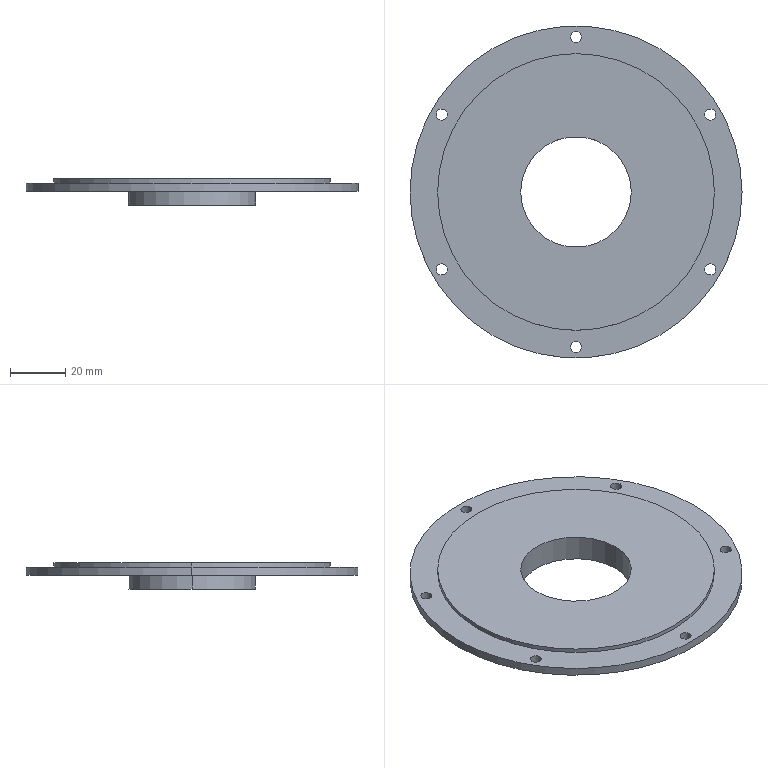Part | SolidWorks | features ICE 1, Revolution 1 | 1 solid | 24 faces | box 120 x 120 x 9.5 mm | volume 41855 mm3 | cylinder 20 | plane 4 | commonest cylinder face diameters 4 x12 40 x2 46 x2 100 x2 120 x2
STEP:
#1=CARTESIAN_POINT('',(2.,56.,-1.5));
#2=VERTEX_POINT('',#1);
#3=CARTESIAN_POINT('',(-2.,56.,-1.5));
#4=VERTEX_POINT('',#3);
#5=CARTESIAN_POINT('',(0.,56.,-1.5));
#6=DIRECTION('',(0.,0.,-1.));
#7=DIRECTION('',(-1.,0.,0.));
#8=AXIS2_PLACEMENT_3D('',#5,#6,#7);
#9=CIRCLE('',#8,2.);
#10=EDGE_CURVE('',#2,#4,#9,.T.);
#11=ORIENTED_EDGE('',*,*,#10,.F.);
#12=CARTESIAN_POINT('',(2.,56.,-4.5));
#13=VERTEX_POINT('',#12);
#14=CARTESIAN_POINT('',(2.,56.,5.5));
#15=DIRECTION('',(0.,0.,-1.));
#16=VECTOR('',#15,1000.);
#17=LINE('',#14,#16);
#18=EDGE_CURVE('',#2,#13,#17,.T.);
#19=ORIENTED_EDGE('',*,*,#18,.T.);
#20=CARTESIAN_POINT('',(-2.,56.,-4.5));
#21=VERTEX_POINT('',#20);
#22=CARTESIAN_POINT('',(0.,56.,-4.5));
#23=DIRECTION('',(0.,0.,-1.));
#24=DIRECTION('',(-1.,0.,0.));
#25=AXIS2_PLACEMENT_3D('',#22,#23,#24);
#26=CIRCLE('',#25,2.);
#27=EDGE_CURVE('',#13,#21,#26,.T.);
#28=ORIENTED_EDGE('',*,*,#27,.T.);
#29=CARTESIAN_POINT('',(-2.,56.,5.5));
#30=DIRECTION('',(0.,0.,-1.));
#31=VECTOR('',#30,1000.);
#32=LINE('',#29,#31);
#33=EDGE_CURVE('',#4,#21,#32,.T.);
#34=ORIENTED_EDGE('',*,*,#33,.F.);
#35=EDGE_LOOP('',(#11,#19,#28,#34));
#36=FACE_OUTER_BOUND('',#35,.T.);
#37=CARTESIAN_POINT('',(0.,56.,5.5));
#38=DIRECTION('',(0.,0.,-1.));
#39=DIRECTION('',(-1.,0.,0.));
#40=AXIS2_PLACEMENT_3D('',#37,#38,#39);
#41=CYLINDRICAL_SURFACE('',#40,2.);
#42=ADVANCED_FACE('',(#36),#41,.F.);
#43=CARTESIAN_POINT('',(-46.497,28.,-1.5));
#44=VERTEX_POINT('',#43);
#45=CARTESIAN_POINT('',(-50.497,28.,-1.5));
#46=VERTEX_POINT('',#45);
#47=CARTESIAN_POINT('',(-48.497,28.,-1.5));
#48=DIRECTION('',(0.,0.,-1.));
#49=DIRECTION('',(-1.,0.,0.));
#50=AXIS2_PLACEMENT_3D('',#47,#48,#49);
#51=CIRCLE('',#50,2.);
#52=EDGE_CURVE('',#44,#46,#51,.T.);
#53=ORIENTED_EDGE('',*,*,#52,.F.);
#54=CARTESIAN_POINT('',(-46.497,28.,-4.5));
#55=VERTEX_POINT('',#54);
#56=CARTESIAN_POINT('',(-46.497,28.,5.5));
#57=DIRECTION('',(0.,0.,-1.));
#58=VECTOR('',#57,1000.);
#59=LINE('',#56,#58);
#60=EDGE_CURVE('',#44,#55,#59,.T.);
#61=ORIENTED_EDGE('',*,*,#60,.T.);
#62=CARTESIAN_POINT('',(-50.497,28.,-4.5));
#63=VERTEX_POINT('',#62);
#64=CARTESIAN_POINT('',(-48.497,28.,-4.5));
#65=DIRECTION('',(0.,0.,-1.));
#66=DIRECTION('',(-1.,0.,0.));
#67=AXIS2_PLACEMENT_3D('',#64,#65,#66);
#68=CIRCLE('',#67,2.);
#69=EDGE_CURVE('',#55,#63,#68,.T.);
#70=ORIENTED_EDGE('',*,*,#69,.T.);
#71=CARTESIAN_POINT('',(-50.497,28.,5.5));
#72=DIRECTION('',(0.,0.,-1.));
#73=VECTOR('',#72,1000.);
#74=LINE('',#71,#73);
#75=EDGE_CURVE('',#46,#63,#74,.T.);
#76=ORIENTED_EDGE('',*,*,#75,.F.);
#77=EDGE_LOOP('',(#53,#61,#70,#76));
#78=FACE_OUTER_BOUND('',#77,.T.);
#79=CARTESIAN_POINT('',(-48.497,28.,5.5));
#80=DIRECTION('',(0.,0.,-1.));
#81=DIRECTION('',(-1.,0.,0.));
#82=AXIS2_PLACEMENT_3D('',#79,#80,#81);
#83=CYLINDRICAL_SURFACE('',#82,2.);
#84=ADVANCED_FACE('',(#78),#83,.F.);
#85=CARTESIAN_POINT('',(-46.497,-28.,-1.5));
#86=VERTEX_POINT('',#85);
#87=CARTESIAN_POINT('',(-50.497,-28.,-1.5));
#88=VERTEX_POINT('',#87);
#89=CARTESIAN_POINT('',(-48.497,-28.,-1.5));
#90=DIRECTION('',(0.,0.,-1.));
#91=DIRECTION('',(-1.,0.,0.));
#92=AXIS2_PLACEMENT_3D('',#89,#90,#91);
#93=CIRCLE('',#92,2.);
#94=EDGE_CURVE('',#86,#88,#93,.T.);
#95=ORIENTED_EDGE('',*,*,#94,.F.);
#96=CARTESIAN_POINT('',(-46.497,-28.,-4.5));
#97=VERTEX_POINT('',#96);
#98=CARTESIAN_POINT('',(-46.497,-28.,5.5));
#99=DIRECTION('',(0.,0.,-1.));
#100=VECTOR('',#99,1000.);
#101=LINE('',#98,#100);
#102=EDGE_CURVE('',#86,#97,#101,.T.);
#103=ORIENTED_EDGE('',*,*,#102,.T.);
#104=CARTESIAN_POINT('',(-50.497,-28.,-4.5));
#105=VERTEX_POINT('',#104);
#106=CARTESIAN_POINT('',(-48.497,-28.,-4.5));
#107=DIRECTION('',(0.,0.,-1.));
#108=DIRECTION('',(-1.,0.,0.));
#109=AXIS2_PLACEMENT_3D('',#106,#107,#108);
#110=CIRCLE('',#109,2.);
#111=EDGE_CURVE('',#97,#105,#110,.T.);
#112=ORIENTED_EDGE('',*,*,#111,.T.);
#113=CARTESIAN_POINT('',(-50.497,-28.,5.5));
#114=DIRECTION('',(0.,0.,-1.));
#115=VECTOR('',#114,1000.);
#116=LINE('',#113,#115);
#117=EDGE_CURVE('',#88,#105,#116,.T.);
#118=ORIENTED_EDGE('',*,*,#117,.F.);
#119=EDGE_LOOP('',(#95,#103,#112,#118));
#120=FACE_OUTER_BOUND('',#119,.T.);
#121=CARTESIAN_POINT('',(-48.497,-28.,5.5));
#122=DIRECTION('',(0.,0.,-1.));
#123=DIRECTION('',(-1.,0.,0.));
#124=AXIS2_PLACEMENT_3D('',#121,#122,#123);
#125=CYLINDRICAL_SURFACE('',#124,2.);
#126=ADVANCED_FACE('',(#120),#125,.F.);
#127=CARTESIAN_POINT('',(2.,-56.,-1.5));
#128=VERTEX_POINT('',#127);
#129=CARTESIAN_POINT('',(-2.,-56.,-1.5));
#130=VERTEX_POINT('',#129);
#131=CARTESIAN_POINT('',(0.,-56.,-1.5));
#132=DIRECTION('',(0.,0.,-1.));
#133=DIRECTION('',(-1.,0.,0.));
#134=AXIS2_PLACEMENT_3D('',#131,#132,#133);
#135=CIRCLE('',#134,2.);
#136=EDGE_CURVE('',#128,#130,#135,.T.);
#137=ORIENTED_EDGE('',*,*,#136,.F.);
#138=CARTESIAN_POINT('',(2.,-56.,-4.5));
#139=VERTEX_POINT('',#138);
#140=CARTESIAN_POINT('',(2.,-56.,5.5));
#141=DIRECTION('',(0.,0.,-1.));
#142=VECTOR('',#141,1000.);
#143=LINE('',#140,#142);
#144=EDGE_CURVE('',#128,#139,#143,.T.);
#145=ORIENTED_EDGE('',*,*,#144,.T.);
#146=CARTESIAN_POINT('',(-2.,-56.,-4.5));
#147=VERTEX_POINT('',#146);
#148=CARTESIAN_POINT('',(0.,-56.,-4.5));
#149=DIRECTION('',(0.,0.,-1.));
#150=DIRECTION('',(-1.,0.,0.));
#151=AXIS2_PLACEMENT_3D('',#148,#149,#150);
#152=CIRCLE('',#151,2.);
#153=EDGE_CURVE('',#139,#147,#152,.T.);
#154=ORIENTED_EDGE('',*,*,#153,.T.);
#155=CARTESIAN_POINT('',(-2.,-56.,5.5));
#156=DIRECTION('',(0.,0.,-1.));
#157=VECTOR('',#156,1000.);
#158=LINE('',#155,#157);
#159=EDGE_CURVE('',#130,#147,#158,.T.);
#160=ORIENTED_EDGE('',*,*,#159,.F.);
#161=EDGE_LOOP('',(#137,#145,#154,#160));
#162=FACE_OUTER_BOUND('',#161,.T.);
#163=CARTESIAN_POINT('',(0.,-56.,5.5));
#164=DIRECTION('',(0.,0.,-1.));
#165=DIRECTION('',(-1.,0.,0.));
#166=AXIS2_PLACEMENT_3D('',#163,#164,#165);
#167=CYLINDRICAL_SURFACE('',#166,2.);
#168=ADVANCED_FACE('',(#162),#167,.F.);
#169=CARTESIAN_POINT('',(50.497,-28.,-1.5));
#170=VERTEX_POINT('',#169);
#171=CARTESIAN_POINT('',(46.497,-28.,-1.5));
#172=VERTEX_POINT('',#171);
#173=CARTESIAN_POINT('',(48.497,-28.,-1.5));
#174=DIRECTION('',(0.,0.,-1.));
#175=DIRECTION('',(-1.,0.,0.));
#176=AXIS2_PLACEMENT_3D('',#173,#174,#175);
#177=CIRCLE('',#176,2.);
#178=EDGE_CURVE('',#170,#172,#177,.T.);
#179=ORIENTED_EDGE('',*,*,#178,.F.);
#180=CARTESIAN_POINT('',(50.497,-28.,-4.5));
#181=VERTEX_POINT('',#180);
#182=CARTESIAN_POINT('',(50.497,-28.,5.5));
#183=DIRECTION('',(0.,0.,-1.));
#184=VECTOR('',#183,1000.);
#185=LINE('',#182,#184);
#186=EDGE_CURVE('',#170,#181,#185,.T.);
#187=ORIENTED_EDGE('',*,*,#186,.T.);
#188=CARTESIAN_POINT('',(46.497,-28.,-4.5));
#189=VERTEX_POINT('',#188);
#190=CARTESIAN_POINT('',(48.497,-28.,-4.5));
#191=DIRECTION('',(0.,0.,-1.));
#192=DIRECTION('',(-1.,0.,0.));
#193=AXIS2_PLACEMENT_3D('',#190,#191,#192);
#194=CIRCLE('',#193,2.);
#195=EDGE_CURVE('',#181,#189,#194,.T.);
#196=ORIENTED_EDGE('',*,*,#195,.T.);
#197=CARTESIAN_POINT('',(46.497,-28.,5.5));
#198=DIRECTION('',(0.,0.,-1.));
#199=VECTOR('',#198,1000.);
#200=LINE('',#197,#199);
#201=EDGE_CURVE('',#172,#189,#200,.T.);
#202=ORIENTED_EDGE('',*,*,#201,.F.);
#203=EDGE_LOOP('',(#179,#187,#196,#202));
#204=FACE_OUTER_BOUND('',#203,.T.);
#205=CARTESIAN_POINT('',(48.497,-28.,5.5));
#206=DIRECTION('',(0.,0.,-1.));
#207=DIRECTION('',(-1.,0.,0.));
#208=AXIS2_PLACEMENT_3D('',#205,#206,#207);
#209=CYLINDRICAL_SURFACE('',#208,2.);
#210=ADVANCED_FACE('',(#204),#209,.F.);
#211=CARTESIAN_POINT('',(50.497,28.,-1.5));
#212=VERTEX_POINT('',#211);
#213=CARTESIAN_POINT('',(46.497,28.,-1.5));
#214=VERTEX_POINT('',#213);
#215=CARTESIAN_POINT('',(48.497,28.,-1.5));
#216=DIRECTION('',(0.,0.,-1.));
#217=DIRECTION('',(-1.,0.,0.));
#218=AXIS2_PLACEMENT_3D('',#215,#216,#217);
#219=CIRCLE('',#218,2.);
#220=EDGE_CURVE('',#212,#214,#219,.T.);
#221=ORIENTED_EDGE('',*,*,#220,.F.);
#222=CARTESIAN_POINT('',(50.497,28.,-4.5));
#223=VERTEX_POINT('',#222);
#224=CARTESIAN_POINT('',(50.497,28.,5.5));
#225=DIRECTION('',(0.,0.,-1.));
#226=VECTOR('',#225,1000.);
#227=LINE('',#224,#226);
#228=EDGE_CURVE('',#212,#223,#227,.T.);
#229=ORIENTED_EDGE('',*,*,#228,.T.);
#230=CARTESIAN_POINT('',(46.497,28.,-4.5));
#231=VERTEX_POINT('',#230);
#232=CARTESIAN_POINT('',(48.497,28.,-4.5));
#233=DIRECTION('',(0.,0.,-1.));
#234=DIRECTION('',(-1.,0.,0.));
#235=AXIS2_PLACEMENT_3D('',#232,#233,#234);
#236=CIRCLE('',#235,2.);
#237=EDGE_CURVE('',#223,#231,#236,.T.);
#238=ORIENTED_EDGE('',*,*,#237,.T.);
#239=CARTESIAN_POINT('',(46.497,28.,5.5));
#240=DIRECTION('',(0.,0.,-1.));
#241=VECTOR('',#240,1000.);
#242=LINE('',#239,#241);
#243=EDGE_CURVE('',#214,#231,#242,.T.);
#244=ORIENTED_EDGE('',*,*,#243,.F.);
#245=EDGE_LOOP('',(#221,#229,#238,#244));
#246=FACE_OUTER_BOUND('',#245,.T.);
#247=CARTESIAN_POINT('',(48.497,28.,5.5));
#248=DIRECTION('',(0.,0.,-1.));
#249=DIRECTION('',(-1.,0.,0.));
#250=AXIS2_PLACEMENT_3D('',#247,#248,#249);
#251=CYLINDRICAL_SURFACE('',#250,2.);
#252=ADVANCED_FACE('',(#246),#251,.F.);
#253=CARTESIAN_POINT('',(-23.,0.,-4.5));
#254=VERTEX_POINT('',#253);
#255=CARTESIAN_POINT('',(23.,0.,-4.5));
#256=VERTEX_POINT('',#255);
#257=CARTESIAN_POINT('',(0.,0.,-4.5));
#258=DIRECTION('',(0.,0.,-1.));
#259=DIRECTION('',(-1.,0.,0.));
#260=AXIS2_PLACEMENT_3D('',#257,#258,#259);
#261=CIRCLE('',#260,23.);
#262=EDGE_CURVE('',#254,#256,#261,.T.);
#263=ORIENTED_EDGE('',*,*,#262,.T.);
#264=CARTESIAN_POINT('',(23.,0.,-9.5));
#265=VERTEX_POINT('',#264);
#266=CARTESIAN_POINT('',(23.,0.,-4.957));
#267=DIRECTION('',(0.,0.,-1.));
#268=VECTOR('',#267,1000.);
#269=LINE('',#266,#268);
#270=EDGE_CURVE('',#256,#265,#269,.T.);
#271=ORIENTED_EDGE('',*,*,#270,.T.);
#272=CARTESIAN_POINT('',(-23.,0.,-9.5));
#273=VERTEX_POINT('',#272);
#274=CARTESIAN_POINT('',(0.,0.,-9.5));
#275=DIRECTION('',(0.,0.,-1.));
#276=DIRECTION('',(-1.,0.,0.));
#277=AXIS2_PLACEMENT_3D('',#274,#275,#276);
#278=CIRCLE('',#277,23.);
#279=EDGE_CURVE('',#273,#265,#278,.T.);
#280=ORIENTED_EDGE('',*,*,#279,.F.);
#281=CARTESIAN_POINT('',(-23.,0.,-4.957));
#282=DIRECTION('',(0.,0.,-1.));
#283=VECTOR('',#282,1000.);
#284=LINE('',#281,#283);
#285=EDGE_CURVE('',#254,#273,#284,.T.);
#286=ORIENTED_EDGE('',*,*,#285,.F.);
#287=EDGE_LOOP('',(#263,#271,#280,#286));
#288=FACE_OUTER_BOUND('',#287,.T.);
#289=CARTESIAN_POINT('',(0.,0.,-4.957));
#290=DIRECTION('',(0.,0.,-1.));
#291=DIRECTION('',(-1.,0.,0.));
#292=AXIS2_PLACEMENT_3D('',#289,#290,#291);
#293=CYLINDRICAL_SURFACE('',#292,23.);
#294=ADVANCED_FACE('',(#288),#293,.T.);
#295=CARTESIAN_POINT('',(-60.,0.,-1.5));
#296=VERTEX_POINT('',#295);
#297=CARTESIAN_POINT('',(60.,0.,-1.5));
#298=VERTEX_POINT('',#297);
#299=CARTESIAN_POINT('',(0.,0.,-1.5));
#300=DIRECTION('',(0.,0.,-1.));
#301=DIRECTION('',(-1.,0.,0.));
#302=AXIS2_PLACEMENT_3D('',#299,#300,#301);
#303=CIRCLE('',#302,60.);
#304=EDGE_CURVE('',#296,#298,#303,.T.);
#305=ORIENTED_EDGE('',*,*,#304,.T.);
#306=CARTESIAN_POINT('',(60.,0.,-4.5));
#307=VERTEX_POINT('',#306);
#308=CARTESIAN_POINT('',(60.,0.,-4.957));
#309=DIRECTION('',(0.,0.,-1.));
#310=VECTOR('',#309,1000.);
#311=LINE('',#308,#310);
#312=EDGE_CURVE('',#298,#307,#311,.T.);
#313=ORIENTED_EDGE('',*,*,#312,.T.);
#314=CARTESIAN_POINT('',(-60.,0.,-4.5));
#315=VERTEX_POINT('',#314);
#316=CARTESIAN_POINT('',(0.,0.,-4.5));
#317=DIRECTION('',(0.,0.,-1.));
#318=DIRECTION('',(-1.,0.,0.));
#319=AXIS2_PLACEMENT_3D('',#316,#317,#318);
#320=CIRCLE('',#319,60.);
#321=EDGE_CURVE('',#315,#307,#320,.T.);
#322=ORIENTED_EDGE('',*,*,#321,.F.);
#323=CARTESIAN_POINT('',(-60.,0.,-4.957));
#324=DIRECTION('',(0.,0.,-1.));
#325=VECTOR('',#324,1000.);
#326=LINE('',#323,#325);
#327=EDGE_CURVE('',#296,#315,#326,.T.);
#328=ORIENTED_EDGE('',*,*,#327,.F.);
#329=EDGE_LOOP('',(#305,#313,#322,#328));
#330=FACE_OUTER_BOUND('',#329,.T.);
#331=CARTESIAN_POINT('',(0.,0.,-4.957));
#332=DIRECTION('',(0.,0.,-1.));
#333=DIRECTION('',(-1.,0.,0.));
#334=AXIS2_PLACEMENT_3D('',#331,#332,#333);
#335=CYLINDRICAL_SURFACE('',#334,60.);
#336=ADVANCED_FACE('',(#330),#335,.T.);
#337=CARTESIAN_POINT('',(-50.,0.,0.));
#338=VERTEX_POINT('',#337);
#339=CARTESIAN_POINT('',(50.,0.,0.));
#340=VERTEX_POINT('',#339);
#341=CARTESIAN_POINT('',(0.,0.,0.));
#342=DIRECTION('',(0.,0.,-1.));
#343=DIRECTION('',(-1.,0.,0.));
#344=AXIS2_PLACEMENT_3D('',#341,#342,#343);
#345=CIRCLE('',#344,50.);
#346=EDGE_CURVE('',#338,#340,#345,.T.);
#347=ORIENTED_EDGE('',*,*,#346,.T.);
#348=CARTESIAN_POINT('',(50.,0.,-1.5));
#349=VERTEX_POINT('',#348);
#350=CARTESIAN_POINT('',(50.,0.,-4.957));
#351=DIRECTION('',(0.,0.,-1.));
#352=VECTOR('',#351,1000.);
#353=LINE('',#350,#352);
#354=EDGE_CURVE('',#340,#349,#353,.T.);
#355=ORIENTED_EDGE('',*,*,#354,.T.);
#356=CARTESIAN_POINT('',(-50.,0.,-1.5));
#357=VERTEX_POINT('',#356);
#358=CARTESIAN_POINT('',(0.,0.,-1.5));
#359=DIRECTION('',(0.,0.,-1.));
#360=DIRECTION('',(-1.,0.,0.));
#361=AXIS2_PLACEMENT_3D('',#358,#359,#360);
#362=CIRCLE('',#361,50.);
#363=EDGE_CURVE('',#357,#349,#362,.T.);
#364=ORIENTED_EDGE('',*,*,#363,.F.);
#365=CARTESIAN_POINT('',(-50.,0.,-4.957));
#366=DIRECTION('',(0.,0.,-1.));
#367=VECTOR('',#366,1000.);
#368=LINE('',#365,#367);
#369=EDGE_CURVE('',#338,#357,#368,.T.);
#370=ORIENTED_EDGE('',*,*,#369,.F.);
#371=EDGE_LOOP('',(#347,#355,#364,#370));
#372=FACE_OUTER_BOUND('',#371,.T.);
#373=CARTESIAN_POINT('',(0.,0.,-4.957));
#374=DIRECTION('',(0.,0.,-1.));
#375=DIRECTION('',(-1.,0.,0.));
#376=AXIS2_PLACEMENT_3D('',#373,#374,#375);
#377=CYLINDRICAL_SURFACE('',#376,50.);
#378=ADVANCED_FACE('',(#372),#377,.T.);
#379=CARTESIAN_POINT('',(20.,0.,0.));
#380=VERTEX_POINT('',#379);
#381=CARTESIAN_POINT('',(-20.,0.,0.));
#382=VERTEX_POINT('',#381);
#383=CARTESIAN_POINT('',(0.,0.,0.));
#384=DIRECTION('',(0.,0.,-1.));
#385=DIRECTION('',(-1.,0.,0.));
#386=AXIS2_PLACEMENT_3D('',#383,#384,#385);
#387=CIRCLE('',#386,20.);
#388=EDGE_CURVE('',#380,#382,#387,.T.);
#389=ORIENTED_EDGE('',*,*,#388,.F.);
#390=CARTESIAN_POINT('',(20.,0.,-9.5));
#391=VERTEX_POINT('',#390);
#392=CARTESIAN_POINT('',(20.,0.,-4.957));
#393=DIRECTION('',(0.,0.,-1.));
#394=VECTOR('',#393,1000.);
#395=LINE('',#392,#394);
#396=EDGE_CURVE('',#380,#391,#395,.T.);
#397=ORIENTED_EDGE('',*,*,#396,.T.);
#398=CARTESIAN_POINT('',(-20.,0.,-9.5));
#399=VERTEX_POINT('',#398);
#400=CARTESIAN_POINT('',(0.,0.,-9.5));
#401=DIRECTION('',(0.,0.,-1.));
#402=DIRECTION('',(-1.,0.,0.));
#403=AXIS2_PLACEMENT_3D('',#400,#401,#402);
#404=CIRCLE('',#403,20.);
#405=EDGE_CURVE('',#391,#399,#404,.T.);
#406=ORIENTED_EDGE('',*,*,#405,.T.);
#407=CARTESIAN_POINT('',(-20.,0.,-4.957));
#408=DIRECTION('',(0.,0.,-1.));
#409=VECTOR('',#408,1000.);
#410=LINE('',#407,#409);
#411=EDGE_CURVE('',#382,#399,#410,.T.);
#412=ORIENTED_EDGE('',*,*,#411,.F.);
#413=EDGE_LOOP('',(#389,#397,#406,#412));
#414=FACE_OUTER_BOUND('',#413,.T.);
#415=CARTESIAN_POINT('',(0.,0.,-4.957));
#416=DIRECTION('',(0.,0.,-1.));
#417=DIRECTION('',(-1.,0.,0.));
#418=AXIS2_PLACEMENT_3D('',#415,#416,#417);
#419=CYLINDRICAL_SURFACE('',#418,20.);
#420=ADVANCED_FACE('',(#414),#419,.F.);
#421=CARTESIAN_POINT('',(0.,0.,-9.5));
#422=DIRECTION('',(0.,0.,-1.));
#423=DIRECTION('',(-1.,0.,0.));
#424=AXIS2_PLACEMENT_3D('',#421,#422,#423);
#425=CIRCLE('',#424,20.);
#426=EDGE_CURVE('',#399,#391,#425,.T.);
#427=ORIENTED_EDGE('',*,*,#426,.F.);
#428=ORIENTED_EDGE('',*,*,#405,.F.);
#429=EDGE_LOOP('',(#427,#428));
#430=FACE_BOUND('',#429,.T.);
#431=ORIENTED_EDGE('',*,*,#279,.T.);
#432=CARTESIAN_POINT('',(0.,0.,-9.5));
#433=DIRECTION('',(0.,0.,-1.));
#434=DIRECTION('',(-1.,0.,0.));
#435=AXIS2_PLACEMENT_3D('',#432,#433,#434);
#436=CIRCLE('',#435,23.);
#437=EDGE_CURVE('',#265,#273,#436,.T.);
#438=ORIENTED_EDGE('',*,*,#437,.T.);
#439=EDGE_LOOP('',(#431,#438));
#440=FACE_OUTER_BOUND('',#439,.T.);
#441=CARTESIAN_POINT('',(23.,0.,-9.5));
#442=DIRECTION('',(0.,0.,1.));
#443=DIRECTION('',(1.,0.,0.));
#444=AXIS2_PLACEMENT_3D('',#441,#442,#443);
#445=PLANE('',#444);
#446=ADVANCED_FACE('',(#430,#440),#445,.F.);
#447=ORIENTED_EDGE('',*,*,#396,.F.);
#448=CARTESIAN_POINT('',(0.,0.,0.));
#449=DIRECTION('',(0.,0.,-1.));
#450=DIRECTION('',(-1.,0.,0.));
#451=AXIS2_PLACEMENT_3D('',#448,#449,#450);
#452=CIRCLE('',#451,20.);
#453=EDGE_CURVE('',#382,#380,#452,.T.);
#454=ORIENTED_EDGE('',*,*,#453,.F.);
#455=ORIENTED_EDGE('',*,*,#411,.T.);
#456=ORIENTED_EDGE('',*,*,#426,.T.);
#457=EDGE_LOOP('',(#447,#454,#455,#456));
#458=FACE_OUTER_BOUND('',#457,.T.);
#459=CARTESIAN_POINT('',(0.,0.,-4.957));
#460=DIRECTION('',(0.,0.,-1.));
#461=DIRECTION('',(-1.,0.,0.));
#462=AXIS2_PLACEMENT_3D('',#459,#460,#461);
#463=CYLINDRICAL_SURFACE('',#462,20.);
#464=ADVANCED_FACE('',(#458),#463,.F.);
#465=ORIENTED_EDGE('',*,*,#346,.F.);
#466=CARTESIAN_POINT('',(0.,0.,0.));
#467=DIRECTION('',(0.,0.,-1.));
#468=DIRECTION('',(-1.,0.,0.));
#469=AXIS2_PLACEMENT_3D('',#466,#467,#468);
#470=CIRCLE('',#469,50.);
#471=EDGE_CURVE('',#340,#338,#470,.T.);
#472=ORIENTED_EDGE('',*,*,#471,.F.);
#473=EDGE_LOOP('',(#465,#472));
#474=FACE_OUTER_BOUND('',#473,.T.);
#475=ORIENTED_EDGE('',*,*,#453,.T.);
#476=ORIENTED_EDGE('',*,*,#388,.T.);
#477=EDGE_LOOP('',(#475,#476));
#478=FACE_BOUND('',#477,.T.);
#479=CARTESIAN_POINT('',(50.,0.,0.));
#480=DIRECTION('',(0.,0.,-1.));
#481=DIRECTION('',(-1.,0.,0.));
#482=AXIS2_PLACEMENT_3D('',#479,#480,#481);
#483=PLANE('',#482);
#484=ADVANCED_FACE('',(#474,#478),#483,.F.);
#485=ORIENTED_EDGE('',*,*,#354,.F.);
#486=ORIENTED_EDGE('',*,*,#471,.T.);
#487=ORIENTED_EDGE('',*,*,#369,.T.);
#488=CARTESIAN_POINT('',(0.,0.,-1.5));
#489=DIRECTION('',(0.,0.,-1.));
#490=DIRECTION('',(-1.,0.,0.));
#491=AXIS2_PLACEMENT_3D('',#488,#489,#490);
#492=CIRCLE('',#491,50.);
#493=EDGE_CURVE('',#349,#357,#492,.T.);
#494=ORIENTED_EDGE('',*,*,#493,.F.);
#495=EDGE_LOOP('',(#485,#486,#487,#494));
#496=FACE_OUTER_BOUND('',#495,.T.);
#497=CARTESIAN_POINT('',(0.,0.,-4.957));
#498=DIRECTION('',(0.,0.,-1.));
#499=DIRECTION('',(-1.,0.,0.));
#500=AXIS2_PLACEMENT_3D('',#497,#498,#499);
#501=CYLINDRICAL_SURFACE('',#500,50.);
#502=ADVANCED_FACE('',(#496),#501,.T.);
#503=CARTESIAN_POINT('',(0.,56.,-1.5));
#504=DIRECTION('',(0.,0.,-1.));
#505=DIRECTION('',(-1.,0.,0.));
#506=AXIS2_PLACEMENT_3D('',#503,#504,#505);
#507=CIRCLE('',#506,2.);
#508=EDGE_CURVE('',#4,#2,#507,.T.);
#509=ORIENTED_EDGE('',*,*,#508,.T.);
#510=ORIENTED_EDGE('',*,*,#10,.T.);
#511=EDGE_LOOP('',(#509,#510));
#512=FACE_BOUND('',#511,.T.);
#513=CARTESIAN_POINT('',(-48.497,28.,-1.5));
#514=DIRECTION('',(0.,0.,-1.));
#515=DIRECTION('',(-1.,0.,0.));
#516=AXIS2_PLACEMENT_3D('',#513,#514,#515);
#517=CIRCLE('',#516,2.);
#518=EDGE_CURVE('',#46,#44,#517,.T.);
#519=ORIENTED_EDGE('',*,*,#518,.T.);
#520=ORIENTED_EDGE('',*,*,#52,.T.);
#521=EDGE_LOOP('',(#519,#520));
#522=FACE_BOUND('',#521,.T.);
#523=CARTESIAN_POINT('',(-48.497,-28.,-1.5));
#524=DIRECTION('',(0.,0.,-1.));
#525=DIRECTION('',(-1.,0.,0.));
#526=AXIS2_PLACEMENT_3D('',#523,#524,#525);
#527=CIRCLE('',#526,2.);
#528=EDGE_CURVE('',#88,#86,#527,.T.);
#529=ORIENTED_EDGE('',*,*,#528,.T.);
#530=ORIENTED_EDGE('',*,*,#94,.T.);
#531=EDGE_LOOP('',(#529,#530));
#532=FACE_BOUND('',#531,.T.);
#533=CARTESIAN_POINT('',(0.,-56.,-1.5));
#534=DIRECTION('',(0.,0.,-1.));
#535=DIRECTION('',(-1.,0.,0.));
#536=AXIS2_PLACEMENT_3D('',#533,#534,#535);
#537=CIRCLE('',#536,2.);
#538=EDGE_CURVE('',#130,#128,#537,.T.);
#539=ORIENTED_EDGE('',*,*,#538,.T.);
#540=ORIENTED_EDGE('',*,*,#136,.T.);
#541=EDGE_LOOP('',(#539,#540));
#542=FACE_BOUND('',#541,.T.);
#543=CARTESIAN_POINT('',(48.497,-28.,-1.5));
#544=DIRECTION('',(0.,0.,-1.));
#545=DIRECTION('',(-1.,0.,0.));
#546=AXIS2_PLACEMENT_3D('',#543,#544,#545);
#547=CIRCLE('',#546,2.);
#548=EDGE_CURVE('',#172,#170,#547,.T.);
#549=ORIENTED_EDGE('',*,*,#548,.T.);
#550=ORIENTED_EDGE('',*,*,#178,.T.);
#551=EDGE_LOOP('',(#549,#550));
#552=FACE_BOUND('',#551,.T.);
#553=CARTESIAN_POINT('',(48.497,28.,-1.5));
#554=DIRECTION('',(0.,0.,-1.));
#555=DIRECTION('',(-1.,0.,0.));
#556=AXIS2_PLACEMENT_3D('',#553,#554,#555);
#557=CIRCLE('',#556,2.);
#558=EDGE_CURVE('',#214,#212,#557,.T.);
#559=ORIENTED_EDGE('',*,*,#558,.T.);
#560=ORIENTED_EDGE('',*,*,#220,.T.);
#561=EDGE_LOOP('',(#559,#560));
#562=FACE_BOUND('',#561,.T.);
#563=ORIENTED_EDGE('',*,*,#304,.F.);
#564=CARTESIAN_POINT('',(0.,0.,-1.5));
#565=DIRECTION('',(0.,0.,-1.));
#566=DIRECTION('',(-1.,0.,0.));
#567=AXIS2_PLACEMENT_3D('',#564,#565,#566);
#568=CIRCLE('',#567,60.);
#569=EDGE_CURVE('',#298,#296,#568,.T.);
#570=ORIENTED_EDGE('',*,*,#569,.F.);
#571=EDGE_LOOP('',(#563,#570));
#572=FACE_OUTER_BOUND('',#571,.T.);
#573=ORIENTED_EDGE('',*,*,#363,.T.);
#574=ORIENTED_EDGE('',*,*,#493,.T.);
#575=EDGE_LOOP('',(#573,#574));
#576=FACE_BOUND('',#575,.T.);
#577=CARTESIAN_POINT('',(50.,0.,-1.5));
#578=DIRECTION('',(0.,0.,-1.));
#579=DIRECTION('',(-1.,0.,0.));
#580=AXIS2_PLACEMENT_3D('',#577,#578,#579);
#581=PLANE('',#580);
#582=ADVANCED_FACE('',(#512,#522,#532,#542,#552,#562,#572,#576),#581,.F.);
#583=ORIENTED_EDGE('',*,*,#312,.F.);
#584=ORIENTED_EDGE('',*,*,#569,.T.);
#585=ORIENTED_EDGE('',*,*,#327,.T.);
#586=CARTESIAN_POINT('',(0.,0.,-4.5));
#587=DIRECTION('',(0.,0.,-1.));
#588=DIRECTION('',(-1.,0.,0.));
#589=AXIS2_PLACEMENT_3D('',#586,#587,#588);
#590=CIRCLE('',#589,60.);
#591=EDGE_CURVE('',#307,#315,#590,.T.);
#592=ORIENTED_EDGE('',*,*,#591,.F.);
#593=EDGE_LOOP('',(#583,#584,#585,#592));
#594=FACE_OUTER_BOUND('',#593,.T.);
#595=CARTESIAN_POINT('',(0.,0.,-4.957));
#596=DIRECTION('',(0.,0.,-1.));
#597=DIRECTION('',(-1.,0.,0.));
#598=AXIS2_PLACEMENT_3D('',#595,#596,#597);
#599=CYLINDRICAL_SURFACE('',#598,60.);
#600=ADVANCED_FACE('',(#594),#599,.T.);
#601=CARTESIAN_POINT('',(0.,56.,-4.5));
#602=DIRECTION('',(0.,0.,-1.));
#603=DIRECTION('',(-1.,0.,0.));
#604=AXIS2_PLACEMENT_3D('',#601,#602,#603);
#605=CIRCLE('',#604,2.);
#606=EDGE_CURVE('',#21,#13,#605,.T.);
#607=ORIENTED_EDGE('',*,*,#606,.F.);
#608=ORIENTED_EDGE('',*,*,#27,.F.);
#609=EDGE_LOOP('',(#607,#608));
#610=FACE_BOUND('',#609,.T.);
#611=CARTESIAN_POINT('',(-48.497,28.,-4.5));
#612=DIRECTION('',(0.,0.,-1.));
#613=DIRECTION('',(-1.,0.,0.));
#614=AXIS2_PLACEMENT_3D('',#611,#612,#613);
#615=CIRCLE('',#614,2.);
#616=EDGE_CURVE('',#63,#55,#615,.T.);
#617=ORIENTED_EDGE('',*,*,#616,.F.);
#618=ORIENTED_EDGE('',*,*,#69,.F.);
#619=EDGE_LOOP('',(#617,#618));
#620=FACE_BOUND('',#619,.T.);
#621=CARTESIAN_POINT('',(-48.497,-28.,-4.5));
#622=DIRECTION('',(0.,0.,-1.));
#623=DIRECTION('',(-1.,0.,0.));
#624=AXIS2_PLACEMENT_3D('',#621,#622,#623);
#625=CIRCLE('',#624,2.);
#626=EDGE_CURVE('',#105,#97,#625,.T.);
#627=ORIENTED_EDGE('',*,*,#626,.F.);
#628=ORIENTED_EDGE('',*,*,#111,.F.);
#629=EDGE_LOOP('',(#627,#628));
#630=FACE_BOUND('',#629,.T.);
#631=CARTESIAN_POINT('',(0.,-56.,-4.5));
#632=DIRECTION('',(0.,0.,-1.));
#633=DIRECTION('',(-1.,0.,0.));
#634=AXIS2_PLACEMENT_3D('',#631,#632,#633);
#635=CIRCLE('',#634,2.);
#636=EDGE_CURVE('',#147,#139,#635,.T.);
#637=ORIENTED_EDGE('',*,*,#636,.F.);
#638=ORIENTED_EDGE('',*,*,#153,.F.);
#639=EDGE_LOOP('',(#637,#638));
#640=FACE_BOUND('',#639,.T.);
#641=CARTESIAN_POINT('',(48.497,-28.,-4.5));
#642=DIRECTION('',(0.,0.,-1.));
#643=DIRECTION('',(-1.,0.,0.));
#644=AXIS2_PLACEMENT_3D('',#641,#642,#643);
#645=CIRCLE('',#644,2.);
#646=EDGE_CURVE('',#189,#181,#645,.T.);
#647=ORIENTED_EDGE('',*,*,#646,.F.);
#648=ORIENTED_EDGE('',*,*,#195,.F.);
#649=EDGE_LOOP('',(#647,#648));
#650=FACE_BOUND('',#649,.T.);
#651=CARTESIAN_POINT('',(48.497,28.,-4.5));
#652=DIRECTION('',(0.,0.,-1.));
#653=DIRECTION('',(-1.,0.,0.));
#654=AXIS2_PLACEMENT_3D('',#651,#652,#653);
#655=CIRCLE('',#654,2.);
#656=EDGE_CURVE('',#231,#223,#655,.T.);
#657=ORIENTED_EDGE('',*,*,#656,.F.);
#658=ORIENTED_EDGE('',*,*,#237,.F.);
#659=EDGE_LOOP('',(#657,#658));
#660=FACE_BOUND('',#659,.T.);
#661=ORIENTED_EDGE('',*,*,#262,.F.);
#662=CARTESIAN_POINT('',(0.,0.,-4.5));
#663=DIRECTION('',(0.,0.,-1.));
#664=DIRECTION('',(-1.,0.,0.));
#665=AXIS2_PLACEMENT_3D('',#662,#663,#664);
#666=CIRCLE('',#665,23.);
#667=EDGE_CURVE('',#256,#254,#666,.T.);
#668=ORIENTED_EDGE('',*,*,#667,.F.);
#669=EDGE_LOOP('',(#661,#668));
#670=FACE_BOUND('',#669,.T.);
#671=ORIENTED_EDGE('',*,*,#321,.T.);
#672=ORIENTED_EDGE('',*,*,#591,.T.);
#673=EDGE_LOOP('',(#671,#672));
#674=FACE_OUTER_BOUND('',#673,.T.);
#675=CARTESIAN_POINT('',(60.,0.,-4.5));
#676=DIRECTION('',(0.,0.,1.));
#677=DIRECTION('',(1.,0.,0.));
#678=AXIS2_PLACEMENT_3D('',#675,#676,#677);
#679=PLANE('',#678);
#680=ADVANCED_FACE('',(#610,#620,#630,#640,#650,#660,#670,#674),#679,.F.);
#681=ORIENTED_EDGE('',*,*,#270,.F.);
#682=ORIENTED_EDGE('',*,*,#667,.T.);
#683=ORIENTED_EDGE('',*,*,#285,.T.);
#684=ORIENTED_EDGE('',*,*,#437,.F.);
#685=EDGE_LOOP('',(#681,#682,#683,#684));
#686=FACE_OUTER_BOUND('',#685,.T.);
#687=CARTESIAN_POINT('',(0.,0.,-4.957));
#688=DIRECTION('',(0.,0.,-1.));
#689=DIRECTION('',(-1.,0.,0.));
#690=AXIS2_PLACEMENT_3D('',#687,#688,#689);
#691=CYLINDRICAL_SURFACE('',#690,23.);
#692=ADVANCED_FACE('',(#686),#691,.T.);
#693=ORIENTED_EDGE('',*,*,#228,.F.);
#694=ORIENTED_EDGE('',*,*,#558,.F.);
#695=ORIENTED_EDGE('',*,*,#243,.T.);
#696=ORIENTED_EDGE('',*,*,#656,.T.);
#697=EDGE_LOOP('',(#693,#694,#695,#696));
#698=FACE_OUTER_BOUND('',#697,.T.);
#699=CARTESIAN_POINT('',(48.497,28.,5.5));
#700=DIRECTION('',(0.,0.,-1.));
#701=DIRECTION('',(-1.,0.,0.));
#702=AXIS2_PLACEMENT_3D('',#699,#700,#701);
#703=CYLINDRICAL_SURFACE('',#702,2.);
#704=ADVANCED_FACE('',(#698),#703,.F.);
#705=ORIENTED_EDGE('',*,*,#186,.F.);
#706=ORIENTED_EDGE('',*,*,#548,.F.);
#707=ORIENTED_EDGE('',*,*,#201,.T.);
#708=ORIENTED_EDGE('',*,*,#646,.T.);
#709=EDGE_LOOP('',(#705,#706,#707,#708));
#710=FACE_OUTER_BOUND('',#709,.T.);
#711=CARTESIAN_POINT('',(48.497,-28.,5.5));
#712=DIRECTION('',(0.,0.,-1.));
#713=DIRECTION('',(-1.,0.,0.));
#714=AXIS2_PLACEMENT_3D('',#711,#712,#713);
#715=CYLINDRICAL_SURFACE('',#714,2.);
#716=ADVANCED_FACE('',(#710),#715,.F.);
#717=ORIENTED_EDGE('',*,*,#144,.F.);
#718=ORIENTED_EDGE('',*,*,#538,.F.);
#719=ORIENTED_EDGE('',*,*,#159,.T.);
#720=ORIENTED_EDGE('',*,*,#636,.T.);
#721=EDGE_LOOP('',(#717,#718,#719,#720));
#722=FACE_OUTER_BOUND('',#721,.T.);
#723=CARTESIAN_POINT('',(0.,-56.,5.5));
#724=DIRECTION('',(0.,0.,-1.));
#725=DIRECTION('',(-1.,0.,0.));
#726=AXIS2_PLACEMENT_3D('',#723,#724,#725);
#727=CYLINDRICAL_SURFACE('',#726,2.);
#728=ADVANCED_FACE('',(#722),#727,.F.);
#729=ORIENTED_EDGE('',*,*,#102,.F.);
#730=ORIENTED_EDGE('',*,*,#528,.F.);
#731=ORIENTED_EDGE('',*,*,#117,.T.);
#732=ORIENTED_EDGE('',*,*,#626,.T.);
#733=EDGE_LOOP('',(#729,#730,#731,#732));
#734=FACE_OUTER_BOUND('',#733,.T.);
#735=CARTESIAN_POINT('',(-48.497,-28.,5.5));
#736=DIRECTION('',(0.,0.,-1.));
#737=DIRECTION('',(-1.,0.,0.));
#738=AXIS2_PLACEMENT_3D('',#735,#736,#737);
#739=CYLINDRICAL_SURFACE('',#738,2.);
#740=ADVANCED_FACE('',(#734),#739,.F.);
#741=ORIENTED_EDGE('',*,*,#60,.F.);
#742=ORIENTED_EDGE('',*,*,#518,.F.);
#743=ORIENTED_EDGE('',*,*,#75,.T.);
#744=ORIENTED_EDGE('',*,*,#616,.T.);
#745=EDGE_LOOP('',(#741,#742,#743,#744));
#746=FACE_OUTER_BOUND('',#745,.T.);
#747=CARTESIAN_POINT('',(-48.497,28.,5.5));
#748=DIRECTION('',(0.,0.,-1.));
#749=DIRECTION('',(-1.,0.,0.));
#750=AXIS2_PLACEMENT_3D('',#747,#748,#749);
#751=CYLINDRICAL_SURFACE('',#750,2.);
#752=ADVANCED_FACE('',(#746),#751,.F.);
#753=ORIENTED_EDGE('',*,*,#18,.F.);
#754=ORIENTED_EDGE('',*,*,#508,.F.);
#755=ORIENTED_EDGE('',*,*,#33,.T.);
#756=ORIENTED_EDGE('',*,*,#606,.T.);
#757=EDGE_LOOP('',(#753,#754,#755,#756));
#758=FACE_OUTER_BOUND('',#757,.T.);
#759=CARTESIAN_POINT('',(0.,56.,5.5));
#760=DIRECTION('',(0.,0.,-1.));
#761=DIRECTION('',(-1.,0.,0.));
#762=AXIS2_PLACEMENT_3D('',#759,#760,#761);
#763=CYLINDRICAL_SURFACE('',#762,2.);
#764=ADVANCED_FACE('',(#758),#763,.F.);
#765=CLOSED_SHELL('',(#42,#84,#126,#168,#210,#252,#294,#336,#378,#420,#446,#464,#484,#502,#582,#600,#680,#692,#704,#716,#728,#740,#752,#764));
#766=MANIFOLD_SOLID_BREP('',#765);
#767=CARTESIAN_POINT('',(0.,0.,0.));
#768=DIRECTION('',(0.,0.,1.));
#769=DIRECTION('',(1.,0.,0.));
#770=AXIS2_PLACEMENT_3D('',#767,#768,#769);
#771=(LENGTH_UNIT()NAMED_UNIT(*)SI_UNIT(.MILLI.,.METRE.));
#772=UNCERTAINTY_MEASURE_WITH_UNIT(LENGTH_MEASURE(0.00001),#771,'','');
#773=(NAMED_UNIT(*)PLANE_ANGLE_UNIT()SI_UNIT($,.RADIAN.));
#774=(NAMED_UNIT(*)SI_UNIT($,.STERADIAN.)SOLID_ANGLE_UNIT());
#775=(GEOMETRIC_REPRESENTATION_CONTEXT(3)GLOBAL_UNCERTAINTY_ASSIGNED_CONTEXT((#772))GLOBAL_UNIT_ASSIGNED_CONTEXT((#771,#773,#774))REPRESENTATION_CONTEXT('',''));
#776=ADVANCED_BREP_SHAPE_REPRESENTATION('',(#766,#770),#775);